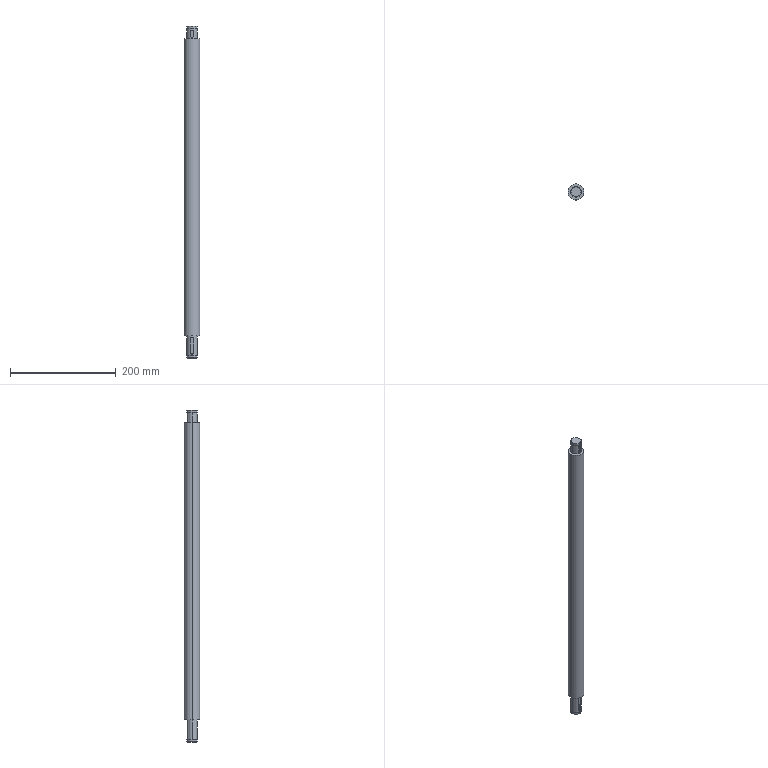Part | SolidWorks | features BaseBody 1 | 1 solid | 36 faces | box 30 x 30 x 627.444 mm | volume 416990 mm3 | cylinder 18 | plane 14 | cone 4 | commonest cylinder face diameters 20 x8 6 x4 18.35 x4 30 x2
STEP:
#1=CARTESIAN_POINT('',(9.,0.,-322.542));
#2=VERTEX_POINT('',#1);
#3=CARTESIAN_POINT('',(-9.,0.,-322.542));
#4=VERTEX_POINT('',#3);
#5=CARTESIAN_POINT('',(0.,0.,-322.542));
#6=DIRECTION('',(0.,0.,1.));
#7=DIRECTION('',(1.,0.,0.));
#8=AXIS2_PLACEMENT_3D('',#5,#6,#7);
#9=CIRCLE('',#8,9.);
#10=EDGE_CURVE('',#2,#4,#9,.T.);
#11=ORIENTED_EDGE('',*,*,#10,.T.);
#12=CARTESIAN_POINT('',(-10.,0.,-321.542));
#13=VERTEX_POINT('',#12);
#14=CARTESIAN_POINT('',(-9.5,0.,-322.042));
#15=DIRECTION('',(-0.7071,0.,0.7071));
#16=VECTOR('',#15,1000.);
#17=LINE('',#14,#16);
#18=EDGE_CURVE('',#4,#13,#17,.T.);
#19=ORIENTED_EDGE('',*,*,#18,.T.);
#20=CARTESIAN_POINT('',(10.,0.,-321.542));
#21=VERTEX_POINT('',#20);
#22=CARTESIAN_POINT('',(0.,0.,-321.542));
#23=DIRECTION('',(0.,0.,-1.));
#24=DIRECTION('',(1.,0.,0.));
#25=AXIS2_PLACEMENT_3D('',#22,#23,#24);
#26=CIRCLE('',#25,10.);
#27=EDGE_CURVE('',#13,#21,#26,.T.);
#28=ORIENTED_EDGE('',*,*,#27,.T.);
#29=CARTESIAN_POINT('',(9.5,0.,-322.042));
#30=DIRECTION('',(0.7071,0.,0.7071));
#31=VECTOR('',#30,1000.);
#32=LINE('',#29,#31);
#33=EDGE_CURVE('',#2,#21,#32,.T.);
#34=ORIENTED_EDGE('',*,*,#33,.F.);
#35=EDGE_LOOP('',(#11,#19,#28,#34));
#36=FACE_OUTER_BOUND('',#35,.T.);
#37=CARTESIAN_POINT('',(0.,0.,-322.042));
#38=DIRECTION('',(0.,0.,1.));
#39=DIRECTION('',(1.,0.,0.));
#40=AXIS2_PLACEMENT_3D('',#37,#38,#39);
#41=CONICAL_SURFACE('',#40,9.5,0.7854);
#42=ADVANCED_FACE('',(#36),#41,.T.);
#43=ORIENTED_EDGE('',*,*,#27,.F.);
#44=CARTESIAN_POINT('',(-10.,0.,-318.542));
#45=VERTEX_POINT('',#44);
#46=CARTESIAN_POINT('',(-10.,0.,-280.932));
#47=DIRECTION('',(0.,0.,1.));
#48=VECTOR('',#47,1000.);
#49=LINE('',#46,#48);
#50=EDGE_CURVE('',#13,#45,#49,.T.);
#51=ORIENTED_EDGE('',*,*,#50,.T.);
#52=CARTESIAN_POINT('',(10.,0.,-318.542));
#53=VERTEX_POINT('',#52);
#54=CARTESIAN_POINT('',(0.,0.,-318.542));
#55=DIRECTION('',(0.,0.,-1.));
#56=DIRECTION('',(1.,0.,0.));
#57=AXIS2_PLACEMENT_3D('',#54,#55,#56);
#58=CIRCLE('',#57,10.);
#59=EDGE_CURVE('',#45,#53,#58,.T.);
#60=ORIENTED_EDGE('',*,*,#59,.T.);
#61=CARTESIAN_POINT('',(10.,0.,-280.932));
#62=DIRECTION('',(0.,0.,1.));
#63=VECTOR('',#62,1000.);
#64=LINE('',#61,#63);
#65=EDGE_CURVE('',#21,#53,#64,.T.);
#66=ORIENTED_EDGE('',*,*,#65,.F.);
#67=EDGE_LOOP('',(#43,#51,#60,#66));
#68=FACE_OUTER_BOUND('',#67,.T.);
#69=CARTESIAN_POINT('',(0.,0.,-280.932));
#70=DIRECTION('',(0.,0.,1.));
#71=DIRECTION('',(1.,0.,0.));
#72=AXIS2_PLACEMENT_3D('',#69,#70,#71);
#73=CYLINDRICAL_SURFACE('',#72,10.);
#74=ADVANCED_FACE('',(#68),#73,.T.);
#75=CARTESIAN_POINT('',(9.175,0.,-317.342));
#76=VERTEX_POINT('',#75);
#77=CARTESIAN_POINT('',(-9.175,0.,-317.342));
#78=VERTEX_POINT('',#77);
#79=CARTESIAN_POINT('',(0.,0.,-317.342));
#80=DIRECTION('',(0.,0.,1.));
#81=DIRECTION('',(1.,0.,0.));
#82=AXIS2_PLACEMENT_3D('',#79,#80,#81);
#83=CIRCLE('',#82,9.175);
#84=EDGE_CURVE('',#76,#78,#83,.T.);
#85=ORIENTED_EDGE('',*,*,#84,.F.);
#86=CARTESIAN_POINT('',(9.175,0.,-318.542));
#87=VERTEX_POINT('',#86);
#88=CARTESIAN_POINT('',(9.175,0.,-317.942));
#89=DIRECTION('',(0.,0.,-1.));
#90=VECTOR('',#89,1000.);
#91=LINE('',#88,#90);
#92=EDGE_CURVE('',#76,#87,#91,.T.);
#93=ORIENTED_EDGE('',*,*,#92,.T.);
#94=CARTESIAN_POINT('',(-9.175,0.,-318.542));
#95=VERTEX_POINT('',#94);
#96=CARTESIAN_POINT('',(0.,0.,-318.542));
#97=DIRECTION('',(0.,0.,1.));
#98=DIRECTION('',(1.,0.,0.));
#99=AXIS2_PLACEMENT_3D('',#96,#97,#98);
#100=CIRCLE('',#99,9.175);
#101=EDGE_CURVE('',#87,#95,#100,.T.);
#102=ORIENTED_EDGE('',*,*,#101,.T.);
#103=CARTESIAN_POINT('',(-9.175,0.,-317.942));
#104=DIRECTION('',(0.,0.,-1.));
#105=VECTOR('',#104,1000.);
#106=LINE('',#103,#105);
#107=EDGE_CURVE('',#78,#95,#106,.T.);
#108=ORIENTED_EDGE('',*,*,#107,.F.);
#109=EDGE_LOOP('',(#85,#93,#102,#108));
#110=FACE_OUTER_BOUND('',#109,.T.);
#111=CARTESIAN_POINT('',(0.,0.,-317.942));
#112=DIRECTION('',(0.,0.,-1.));
#113=DIRECTION('',(-1.,0.,0.));
#114=AXIS2_PLACEMENT_3D('',#111,#112,#113);
#115=CYLINDRICAL_SURFACE('',#114,9.175);
#116=ADVANCED_FACE('',(#110),#115,.T.);
#117=CARTESIAN_POINT('',(10.,0.,-317.342));
#118=VERTEX_POINT('',#117);
#119=CARTESIAN_POINT('',(-10.,0.,-317.342));
#120=VERTEX_POINT('',#119);
#121=CARTESIAN_POINT('',(0.,0.,-317.342));
#122=DIRECTION('',(0.,0.,1.));
#123=DIRECTION('',(1.,0.,0.));
#124=AXIS2_PLACEMENT_3D('',#121,#122,#123);
#125=CIRCLE('',#124,10.);
#126=EDGE_CURVE('',#118,#120,#125,.T.);
#127=ORIENTED_EDGE('',*,*,#126,.T.);
#128=CARTESIAN_POINT('',(-10.,0.,-280.932));
#129=VERTEX_POINT('',#128);
#130=CARTESIAN_POINT('',(-10.,0.,-280.932));
#131=DIRECTION('',(0.,0.,1.));
#132=VECTOR('',#131,1000.);
#133=LINE('',#130,#132);
#134=EDGE_CURVE('',#120,#129,#133,.T.);
#135=ORIENTED_EDGE('',*,*,#134,.T.);
#136=CARTESIAN_POINT('',(10.,0.,-280.932));
#137=VERTEX_POINT('',#136);
#138=CARTESIAN_POINT('',(0.,0.,-280.932));
#139=DIRECTION('',(0.,0.,1.));
#140=DIRECTION('',(1.,0.,0.));
#141=AXIS2_PLACEMENT_3D('',#138,#139,#140);
#142=CIRCLE('',#141,10.);
#143=EDGE_CURVE('',#137,#129,#142,.T.);
#144=ORIENTED_EDGE('',*,*,#143,.F.);
#145=CARTESIAN_POINT('',(10.,0.,-280.932));
#146=DIRECTION('',(0.,0.,1.));
#147=VECTOR('',#146,1000.);
#148=LINE('',#145,#147);
#149=EDGE_CURVE('',#118,#137,#148,.T.);
#150=ORIENTED_EDGE('',*,*,#149,.F.);
#151=EDGE_LOOP('',(#127,#135,#144,#150));
#152=FACE_OUTER_BOUND('',#151,.T.);
#153=CARTESIAN_POINT('',(0.,0.,-280.932));
#154=DIRECTION('',(0.,0.,1.));
#155=DIRECTION('',(1.,0.,0.));
#156=AXIS2_PLACEMENT_3D('',#153,#154,#155);
#157=CYLINDRICAL_SURFACE('',#156,10.);
#158=ADVANCED_FACE('',(#152),#157,.T.);
#159=CARTESIAN_POINT('',(-9.5,0.,304.902));
#160=VERTEX_POINT('',#159);
#161=CARTESIAN_POINT('',(9.5,0.,304.902));
#162=VERTEX_POINT('',#161);
#163=CARTESIAN_POINT('',(0.,0.,304.902));
#164=DIRECTION('',(0.,0.,-1.));
#165=DIRECTION('',(-1.,0.,0.));
#166=AXIS2_PLACEMENT_3D('',#163,#164,#165);
#167=CIRCLE('',#166,9.5);
#168=EDGE_CURVE('',#160,#162,#167,.T.);
#169=ORIENTED_EDGE('',*,*,#168,.T.);
#170=CARTESIAN_POINT('',(10.,0.,304.402));
#171=VERTEX_POINT('',#170);
#172=CARTESIAN_POINT('',(9.75,0.,304.652));
#173=DIRECTION('',(0.7071,0.,-0.7071));
#174=VECTOR('',#173,1000.);
#175=LINE('',#172,#174);
#176=EDGE_CURVE('',#162,#171,#175,.T.);
#177=ORIENTED_EDGE('',*,*,#176,.T.);
#178=CARTESIAN_POINT('',(-10.,0.,304.402));
#179=VERTEX_POINT('',#178);
#180=CARTESIAN_POINT('',(0.,0.,304.402));
#181=DIRECTION('',(0.,0.,1.));
#182=DIRECTION('',(-1.,0.,0.));
#183=AXIS2_PLACEMENT_3D('',#180,#181,#182);
#184=CIRCLE('',#183,10.);
#185=EDGE_CURVE('',#171,#179,#184,.T.);
#186=ORIENTED_EDGE('',*,*,#185,.T.);
#187=CARTESIAN_POINT('',(-9.75,0.,304.652));
#188=DIRECTION('',(-0.7071,0.,-0.7071));
#189=VECTOR('',#188,1000.);
#190=LINE('',#187,#189);
#191=EDGE_CURVE('',#160,#179,#190,.T.);
#192=ORIENTED_EDGE('',*,*,#191,.F.);
#193=EDGE_LOOP('',(#169,#177,#186,#192));
#194=FACE_OUTER_BOUND('',#193,.T.);
#195=CARTESIAN_POINT('',(0.,0.,304.652));
#196=DIRECTION('',(0.,0.,-1.));
#197=DIRECTION('',(-1.,0.,0.));
#198=AXIS2_PLACEMENT_3D('',#195,#196,#197);
#199=CONICAL_SURFACE('',#198,9.75,0.7854);
#200=ADVANCED_FACE('',(#194),#199,.T.);
#201=ORIENTED_EDGE('',*,*,#185,.F.);
#202=CARTESIAN_POINT('',(10.,0.,300.902));
#203=VERTEX_POINT('',#202);
#204=CARTESIAN_POINT('',(10.,0.,280.932));
#205=DIRECTION('',(0.,0.,-1.));
#206=VECTOR('',#205,1000.);
#207=LINE('',#204,#206);
#208=EDGE_CURVE('',#171,#203,#207,.T.);
#209=ORIENTED_EDGE('',*,*,#208,.T.);
#210=CARTESIAN_POINT('',(-10.,0.,300.902));
#211=VERTEX_POINT('',#210);
#212=CARTESIAN_POINT('',(0.,0.,300.902));
#213=DIRECTION('',(0.,0.,1.));
#214=DIRECTION('',(-1.,0.,0.));
#215=AXIS2_PLACEMENT_3D('',#212,#213,#214);
#216=CIRCLE('',#215,10.);
#217=EDGE_CURVE('',#203,#211,#216,.T.);
#218=ORIENTED_EDGE('',*,*,#217,.T.);
#219=CARTESIAN_POINT('',(-10.,0.,280.932));
#220=DIRECTION('',(0.,0.,-1.));
#221=VECTOR('',#220,1000.);
#222=LINE('',#219,#221);
#223=EDGE_CURVE('',#179,#211,#222,.T.);
#224=ORIENTED_EDGE('',*,*,#223,.F.);
#225=EDGE_LOOP('',(#201,#209,#218,#224));
#226=FACE_OUTER_BOUND('',#225,.T.);
#227=CARTESIAN_POINT('',(0.,0.,280.932));
#228=DIRECTION('',(0.,0.,-1.));
#229=DIRECTION('',(-1.,0.,0.));
#230=AXIS2_PLACEMENT_3D('',#227,#228,#229);
#231=CYLINDRICAL_SURFACE('',#230,10.);
#232=ADVANCED_FACE('',(#226),#231,.T.);
#233=CARTESIAN_POINT('',(-9.175,0.,299.702));
#234=VERTEX_POINT('',#233);
#235=CARTESIAN_POINT('',(9.175,0.,299.702));
#236=VERTEX_POINT('',#235);
#237=CARTESIAN_POINT('',(0.,0.,299.702));
#238=DIRECTION('',(0.,0.,-1.));
#239=DIRECTION('',(1.,0.,0.));
#240=AXIS2_PLACEMENT_3D('',#237,#238,#239);
#241=CIRCLE('',#240,9.175);
#242=EDGE_CURVE('',#234,#236,#241,.T.);
#243=ORIENTED_EDGE('',*,*,#242,.F.);
#244=CARTESIAN_POINT('',(-9.175,0.,300.902));
#245=VERTEX_POINT('',#244);
#246=CARTESIAN_POINT('',(-9.175,0.,300.302));
#247=DIRECTION('',(0.,0.,1.));
#248=VECTOR('',#247,1000.);
#249=LINE('',#246,#248);
#250=EDGE_CURVE('',#234,#245,#249,.T.);
#251=ORIENTED_EDGE('',*,*,#250,.T.);
#252=CARTESIAN_POINT('',(9.175,0.,300.902));
#253=VERTEX_POINT('',#252);
#254=CARTESIAN_POINT('',(0.,0.,300.902));
#255=DIRECTION('',(0.,0.,-1.));
#256=DIRECTION('',(1.,0.,0.));
#257=AXIS2_PLACEMENT_3D('',#254,#255,#256);
#258=CIRCLE('',#257,9.175);
#259=EDGE_CURVE('',#245,#253,#258,.T.);
#260=ORIENTED_EDGE('',*,*,#259,.T.);
#261=CARTESIAN_POINT('',(9.175,0.,300.302));
#262=DIRECTION('',(0.,0.,1.));
#263=VECTOR('',#262,1000.);
#264=LINE('',#261,#263);
#265=EDGE_CURVE('',#236,#253,#264,.T.);
#266=ORIENTED_EDGE('',*,*,#265,.F.);
#267=EDGE_LOOP('',(#243,#251,#260,#266));
#268=FACE_OUTER_BOUND('',#267,.T.);
#269=CARTESIAN_POINT('',(0.,0.,300.302));
#270=DIRECTION('',(0.,0.,1.));
#271=DIRECTION('',(1.,0.,0.));
#272=AXIS2_PLACEMENT_3D('',#269,#270,#271);
#273=CYLINDRICAL_SURFACE('',#272,9.175);
#274=ADVANCED_FACE('',(#268),#273,.T.);
#275=CARTESIAN_POINT('',(-10.,0.,299.702));
#276=VERTEX_POINT('',#275);
#277=CARTESIAN_POINT('',(10.,0.,299.702));
#278=VERTEX_POINT('',#277);
#279=CARTESIAN_POINT('',(0.,0.,299.702));
#280=DIRECTION('',(0.,0.,-1.));
#281=DIRECTION('',(-1.,0.,0.));
#282=AXIS2_PLACEMENT_3D('',#279,#280,#281);
#283=CIRCLE('',#282,10.);
#284=EDGE_CURVE('',#276,#278,#283,.T.);
#285=ORIENTED_EDGE('',*,*,#284,.T.);
#286=CARTESIAN_POINT('',(10.,0.,280.932));
#287=VERTEX_POINT('',#286);
#288=CARTESIAN_POINT('',(10.,0.,280.932));
#289=DIRECTION('',(0.,0.,-1.));
#290=VECTOR('',#289,1000.);
#291=LINE('',#288,#290);
#292=EDGE_CURVE('',#278,#287,#291,.T.);
#293=ORIENTED_EDGE('',*,*,#292,.T.);
#294=CARTESIAN_POINT('',(-10.,0.,280.932));
#295=VERTEX_POINT('',#294);
#296=CARTESIAN_POINT('',(0.,0.,280.932));
#297=DIRECTION('',(0.,0.,-1.));
#298=DIRECTION('',(-1.,0.,0.));
#299=AXIS2_PLACEMENT_3D('',#296,#297,#298);
#300=CIRCLE('',#299,10.);
#301=EDGE_CURVE('',#295,#287,#300,.T.);
#302=ORIENTED_EDGE('',*,*,#301,.F.);
#303=CARTESIAN_POINT('',(-10.,0.,280.932));
#304=DIRECTION('',(0.,0.,-1.));
#305=VECTOR('',#304,1000.);
#306=LINE('',#303,#305);
#307=EDGE_CURVE('',#276,#295,#306,.T.);
#308=ORIENTED_EDGE('',*,*,#307,.F.);
#309=EDGE_LOOP('',(#285,#293,#302,#308));
#310=FACE_OUTER_BOUND('',#309,.T.);
#311=CARTESIAN_POINT('',(0.,0.,280.932));
#312=DIRECTION('',(0.,0.,-1.));
#313=DIRECTION('',(-1.,0.,0.));
#314=AXIS2_PLACEMENT_3D('',#311,#312,#313);
#315=CYLINDRICAL_SURFACE('',#314,10.);
#316=ADVANCED_FACE('',(#310),#315,.T.);
#317=CARTESIAN_POINT('',(15.,0.,280.932));
#318=VERTEX_POINT('',#317);
#319=CARTESIAN_POINT('',(-15.,0.,280.932));
#320=VERTEX_POINT('',#319);
#321=CARTESIAN_POINT('',(0.,0.,280.932));
#322=DIRECTION('',(0.,0.,1.));
#323=DIRECTION('',(-1.,0.,0.));
#324=AXIS2_PLACEMENT_3D('',#321,#322,#323);
#325=CIRCLE('',#324,15.);
#326=EDGE_CURVE('',#318,#320,#325,.T.);
#327=ORIENTED_EDGE('',*,*,#326,.F.);
#328=CARTESIAN_POINT('',(15.,0.,-280.932));
#329=VERTEX_POINT('',#328);
#330=CARTESIAN_POINT('',(15.,0.,0.));
#331=DIRECTION('',(0.,0.,-1.));
#332=VECTOR('',#331,1000.);
#333=LINE('',#330,#332);
#334=EDGE_CURVE('',#318,#329,#333,.T.);
#335=ORIENTED_EDGE('',*,*,#334,.T.);
#336=CARTESIAN_POINT('',(-15.,0.,-280.932));
#337=VERTEX_POINT('',#336);
#338=CARTESIAN_POINT('',(0.,0.,-280.932));
#339=DIRECTION('',(0.,0.,-1.));
#340=DIRECTION('',(-1.,0.,0.));
#341=AXIS2_PLACEMENT_3D('',#338,#339,#340);
#342=CIRCLE('',#341,15.);
#343=EDGE_CURVE('',#337,#329,#342,.T.);
#344=ORIENTED_EDGE('',*,*,#343,.F.);
#345=CARTESIAN_POINT('',(-15.,0.,0.));
#346=DIRECTION('',(0.,0.,-1.));
#347=VECTOR('',#346,1000.);
#348=LINE('',#345,#347);
#349=EDGE_CURVE('',#320,#337,#348,.T.);
#350=ORIENTED_EDGE('',*,*,#349,.F.);
#351=EDGE_LOOP('',(#327,#335,#344,#350));
#352=FACE_OUTER_BOUND('',#351,.T.);
#353=CARTESIAN_POINT('',(0.,0.,0.));
#354=DIRECTION('',(0.,0.,-1.));
#355=DIRECTION('',(-1.,0.,0.));
#356=AXIS2_PLACEMENT_3D('',#353,#354,#355);
#357=CYLINDRICAL_SURFACE('',#356,15.);
#358=ADVANCED_FACE('',(#352),#357,.T.);
#359=ORIENTED_EDGE('',*,*,#10,.F.);
#360=CARTESIAN_POINT('',(0.,0.,-322.542));
#361=DIRECTION('',(0.,0.,1.));
#362=DIRECTION('',(1.,0.,0.));
#363=AXIS2_PLACEMENT_3D('',#360,#361,#362);
#364=CIRCLE('',#363,9.);
#365=EDGE_CURVE('',#4,#2,#364,.T.);
#366=ORIENTED_EDGE('',*,*,#365,.F.);
#367=EDGE_LOOP('',(#359,#366));
#368=FACE_OUTER_BOUND('',#367,.T.);
#369=CARTESIAN_POINT('',(0.,0.,-322.542));
#370=DIRECTION('',(0.,0.,1.));
#371=DIRECTION('',(1.,0.,0.));
#372=AXIS2_PLACEMENT_3D('',#369,#370,#371);
#373=PLANE('',#372);
#374=ADVANCED_FACE('',(#368),#373,.F.);
#375=CARTESIAN_POINT('',(0.,0.,-317.342));
#376=DIRECTION('',(0.,0.,1.));
#377=DIRECTION('',(1.,0.,0.));
#378=AXIS2_PLACEMENT_3D('',#375,#376,#377);
#379=CIRCLE('',#378,9.175);
#380=EDGE_CURVE('',#78,#76,#379,.T.);
#381=ORIENTED_EDGE('',*,*,#380,.T.);
#382=ORIENTED_EDGE('',*,*,#84,.T.);
#383=EDGE_LOOP('',(#381,#382));
#384=FACE_BOUND('',#383,.T.);
#385=ORIENTED_EDGE('',*,*,#126,.F.);
#386=CARTESIAN_POINT('',(0.,0.,-317.342));
#387=DIRECTION('',(0.,0.,1.));
#388=DIRECTION('',(1.,0.,0.));
#389=AXIS2_PLACEMENT_3D('',#386,#387,#388);
#390=CIRCLE('',#389,10.);
#391=EDGE_CURVE('',#120,#118,#390,.T.);
#392=ORIENTED_EDGE('',*,*,#391,.F.);
#393=EDGE_LOOP('',(#385,#392));
#394=FACE_OUTER_BOUND('',#393,.T.);
#395=CARTESIAN_POINT('',(-9.175,0.,-317.342));
#396=DIRECTION('',(0.,0.,1.));
#397=DIRECTION('',(1.,0.,0.));
#398=AXIS2_PLACEMENT_3D('',#395,#396,#397);
#399=PLANE('',#398);
#400=ADVANCED_FACE('',(#384,#394),#399,.F.);
#401=CARTESIAN_POINT('',(0.,0.,-318.542));
#402=DIRECTION('',(0.,0.,1.));
#403=DIRECTION('',(1.,0.,0.));
#404=AXIS2_PLACEMENT_3D('',#401,#402,#403);
#405=CIRCLE('',#404,9.175);
#406=EDGE_CURVE('',#95,#87,#405,.T.);
#407=ORIENTED_EDGE('',*,*,#406,.F.);
#408=ORIENTED_EDGE('',*,*,#101,.F.);
#409=EDGE_LOOP('',(#407,#408));
#410=FACE_BOUND('',#409,.T.);
#411=CARTESIAN_POINT('',(0.,0.,-318.542));
#412=DIRECTION('',(0.,0.,-1.));
#413=DIRECTION('',(1.,0.,0.));
#414=AXIS2_PLACEMENT_3D('',#411,#412,#413);
#415=CIRCLE('',#414,10.);
#416=EDGE_CURVE('',#53,#45,#415,.T.);
#417=ORIENTED_EDGE('',*,*,#416,.F.);
#418=ORIENTED_EDGE('',*,*,#59,.F.);
#419=EDGE_LOOP('',(#417,#418));
#420=FACE_OUTER_BOUND('',#419,.T.);
#421=CARTESIAN_POINT('',(-14.987,0.,-318.542));
#422=DIRECTION('',(0.,0.,-1.));
#423=DIRECTION('',(-1.,0.,0.));
#424=AXIS2_PLACEMENT_3D('',#421,#422,#423);
#425=PLANE('',#424);
#426=ADVANCED_FACE('',(#410,#420),#425,.F.);
#427=CARTESIAN_POINT('',(3.,-9.539,-286.137));
#428=VERTEX_POINT('',#427);
#429=CARTESIAN_POINT('',(3.,-9.539,-312.137));
#430=VERTEX_POINT('',#429);
#431=CARTESIAN_POINT('',(3.,-9.539,-280.932));
#432=DIRECTION('',(0.,0.,-1.));
#433=VECTOR('',#432,1000.);
#434=LINE('',#431,#433);
#435=EDGE_CURVE('',#428,#430,#434,.T.);
#436=ORIENTED_EDGE('',*,*,#435,.F.);
#437=CARTESIAN_POINT('',(3.,-7.5,-286.137));
#438=VERTEX_POINT('',#437);
#439=CARTESIAN_POINT('',(3.,-10.,-286.137));
#440=DIRECTION('',(0.,1.,0.));
#441=VECTOR('',#440,1000.);
#442=LINE('',#439,#441);
#443=EDGE_CURVE('',#428,#438,#442,.T.);
#444=ORIENTED_EDGE('',*,*,#443,.T.);
#445=CARTESIAN_POINT('',(3.,-7.5,-312.137));
#446=VERTEX_POINT('',#445);
#447=CARTESIAN_POINT('',(3.,-7.5,-286.137));
#448=DIRECTION('',(0.,0.,-1.));
#449=VECTOR('',#448,1000.);
#450=LINE('',#447,#449);
#451=EDGE_CURVE('',#438,#446,#450,.T.);
#452=ORIENTED_EDGE('',*,*,#451,.T.);
#453=CARTESIAN_POINT('',(3.,-10.,-312.137));
#454=DIRECTION('',(0.,1.,0.));
#455=VECTOR('',#454,1000.);
#456=LINE('',#453,#455);
#457=EDGE_CURVE('',#430,#446,#456,.T.);
#458=ORIENTED_EDGE('',*,*,#457,.F.);
#459=EDGE_LOOP('',(#436,#444,#452,#458));
#460=FACE_OUTER_BOUND('',#459,.T.);
#461=CARTESIAN_POINT('',(3.,-10.,-286.137));
#462=DIRECTION('',(1.,0.,0.));
#463=DIRECTION('',(0.,0.,-1.));
#464=AXIS2_PLACEMENT_3D('',#461,#462,#463);
#465=PLANE('',#464);
#466=ADVANCED_FACE('',(#460),#465,.F.);
#467=CARTESIAN_POINT('',(-3.,-9.539,-312.137));
#468=VERTEX_POINT('',#467);
#469=CARTESIAN_POINT('',(3.,-9.539,-312.137));
#470=CARTESIAN_POINT('',(3.,-9.539,-312.336));
#471=CARTESIAN_POINT('',(2.98,-9.546,-312.532));
#472=CARTESIAN_POINT('',(2.904,-9.569,-312.917));
#473=CARTESIAN_POINT('',(2.845,-9.587,-313.108));
#474=CARTESIAN_POINT('',(2.695,-9.63,-313.47));
#475=CARTESIAN_POINT('',(2.602,-9.656,-313.642));
#476=CARTESIAN_POINT('',(2.385,-9.712,-313.967));
#477=CARTESIAN_POINT('',(2.259,-9.742,-314.12));
#478=CARTESIAN_POINT('',(1.847,-9.832,-314.533));
#479=CARTESIAN_POINT('',(1.515,-9.891,-314.756));
#480=CARTESIAN_POINT('',(0.9743,-9.954,-314.981));
#481=CARTESIAN_POINT('',(0.7844,-9.971,-315.039));
#482=CARTESIAN_POINT('',(0.396,-9.994,-315.117));
#483=CARTESIAN_POINT('',(0.1993,-10.,-315.137));
#484=CARTESIAN_POINT('',(-0.1994,-10.,-315.137));
#485=CARTESIAN_POINT('',(-0.3951,-9.994,-315.117));
#486=CARTESIAN_POINT('',(-0.7799,-9.971,-315.04));
#487=CARTESIAN_POINT('',(-0.971,-9.954,-314.982));
#488=CARTESIAN_POINT('',(-1.334,-9.912,-314.831));
#489=CARTESIAN_POINT('',(-1.505,-9.887,-314.739));
#490=CARTESIAN_POINT('',(-1.831,-9.832,-314.522));
#491=CARTESIAN_POINT('',(-1.984,-9.802,-314.396));
#492=CARTESIAN_POINT('',(-2.396,-9.713,-313.984));
#493=CARTESIAN_POINT('',(-2.619,-9.652,-313.651));
#494=CARTESIAN_POINT('',(-2.844,-9.587,-313.111));
#495=CARTESIAN_POINT('',(-2.902,-9.57,-312.921));
#496=CARTESIAN_POINT('',(-2.98,-9.546,-312.533));
#497=CARTESIAN_POINT('',(-3.,-9.539,-312.336));
#498=CARTESIAN_POINT('',(-3.,-9.539,-312.137));
#499=B_SPLINE_CURVE_WITH_KNOTS('',3,(#469,#470,#471,#472,#473,#474,#475,#476,#477,#478,#479,#480,#481,#482,#483,#484,#485,#486,#487,#488,#489,#490,#491,#492,#493,#494,#495,#496,#497,#498),.UNSPECIFIED.,.F.,.F.,(4,2,2,2,2,2,2,2,2,2,2,2,2,2,4),(0.,0.0005892,0.001178,0.001768,0.002357,0.003535,0.004125,0.004714,0.005303,0.005892,0.006482,0.007071,0.008249,0.008838,0.009428),.UNSPECIFIED.);
#500=EDGE_CURVE('',#430,#468,#499,.T.);
#501=ORIENTED_EDGE('',*,*,#500,.F.);
#502=ORIENTED_EDGE('',*,*,#457,.T.);
#503=CARTESIAN_POINT('',(-3.,-7.5,-312.137));
#504=VERTEX_POINT('',#503);
#505=CARTESIAN_POINT('',(0.,-7.5,-312.137));
#506=DIRECTION('',(0.,1.,0.));
#507=DIRECTION('',(1.,0.,0.));
#508=AXIS2_PLACEMENT_3D('',#505,#506,#507);
#509=CIRCLE('',#508,3.);
#510=EDGE_CURVE('',#446,#504,#509,.T.);
#511=ORIENTED_EDGE('',*,*,#510,.T.);
#512=CARTESIAN_POINT('',(-3.,-10.,-312.137));
#513=DIRECTION('',(0.,1.,0.));
#514=VECTOR('',#513,1000.);
#515=LINE('',#512,#514);
#516=EDGE_CURVE('',#468,#504,#515,.T.);
#517=ORIENTED_EDGE('',*,*,#516,.F.);
#518=EDGE_LOOP('',(#501,#502,#511,#517));
#519=FACE_OUTER_BOUND('',#518,.T.);
#520=CARTESIAN_POINT('',(0.,-10.,-312.137));
#521=DIRECTION('',(0.,-1.,0.));
#522=DIRECTION('',(1.,0.,0.));
#523=AXIS2_PLACEMENT_3D('',#520,#521,#522);
#524=CYLINDRICAL_SURFACE('',#523,3.);
#525=ADVANCED_FACE('',(#519),#524,.F.);
#526=CARTESIAN_POINT('',(-3.,-9.539,-286.137));
#527=VERTEX_POINT('',#526);
#528=CARTESIAN_POINT('',(-3.,-9.539,-280.932));
#529=DIRECTION('',(0.,0.,1.));
#530=VECTOR('',#529,1000.);
#531=LINE('',#528,#530);
#532=EDGE_CURVE('',#468,#527,#531,.T.);
#533=ORIENTED_EDGE('',*,*,#532,.F.);
#534=ORIENTED_EDGE('',*,*,#516,.T.);
#535=CARTESIAN_POINT('',(-3.,-7.5,-286.137));
#536=VERTEX_POINT('',#535);
#537=CARTESIAN_POINT('',(-3.,-7.5,-312.137));
#538=DIRECTION('',(0.,0.,1.));
#539=VECTOR('',#538,1000.);
#540=LINE('',#537,#539);
#541=EDGE_CURVE('',#504,#536,#540,.T.);
#542=ORIENTED_EDGE('',*,*,#541,.T.);
#543=CARTESIAN_POINT('',(-3.,-10.,-286.137));
#544=DIRECTION('',(0.,1.,0.));
#545=VECTOR('',#544,1000.);
#546=LINE('',#543,#545);
#547=EDGE_CURVE('',#527,#536,#546,.T.);
#548=ORIENTED_EDGE('',*,*,#547,.F.);
#549=EDGE_LOOP('',(#533,#534,#542,#548));
#550=FACE_OUTER_BOUND('',#549,.T.);
#551=CARTESIAN_POINT('',(-3.,-10.,-312.137));
#552=DIRECTION('',(-1.,0.,0.));
#553=DIRECTION('',(0.,0.,1.));
#554=AXIS2_PLACEMENT_3D('',#551,#552,#553);
#555=PLANE('',#554);
#556=ADVANCED_FACE('',(#550),#555,.F.);
#557=ORIENTED_EDGE('',*,*,#443,.F.);
#558=CARTESIAN_POINT('',(-3.,-9.539,-286.137));
#559=CARTESIAN_POINT('',(-3.,-9.539,-285.938));
#560=CARTESIAN_POINT('',(-2.98,-9.546,-285.742));
#561=CARTESIAN_POINT('',(-2.904,-9.569,-285.357));
#562=CARTESIAN_POINT('',(-2.845,-9.587,-285.166));
#563=CARTESIAN_POINT('',(-2.695,-9.63,-284.804));
#564=CARTESIAN_POINT('',(-2.602,-9.656,-284.632));
#565=CARTESIAN_POINT('',(-2.385,-9.712,-284.307));
#566=CARTESIAN_POINT('',(-2.259,-9.742,-284.154));
#567=CARTESIAN_POINT('',(-1.847,-9.832,-283.741));
#568=CARTESIAN_POINT('',(-1.515,-9.891,-283.518));
#569=CARTESIAN_POINT('',(-0.9743,-9.954,-283.293));
#570=CARTESIAN_POINT('',(-0.7844,-9.971,-283.235));
#571=CARTESIAN_POINT('',(-0.396,-9.994,-283.157));
#572=CARTESIAN_POINT('',(-0.1993,-10.,-283.137));
#573=CARTESIAN_POINT('',(0.1994,-10.,-283.137));
#574=CARTESIAN_POINT('',(0.3951,-9.994,-283.157));
#575=CARTESIAN_POINT('',(0.7799,-9.971,-283.234));
#576=CARTESIAN_POINT('',(0.971,-9.954,-283.292));
#577=CARTESIAN_POINT('',(1.334,-9.912,-283.443));
#578=CARTESIAN_POINT('',(1.505,-9.887,-283.535));
#579=CARTESIAN_POINT('',(1.831,-9.832,-283.752));
#580=CARTESIAN_POINT('',(1.984,-9.802,-283.878));
#581=CARTESIAN_POINT('',(2.396,-9.713,-284.29));
#582=CARTESIAN_POINT('',(2.619,-9.652,-284.623));
#583=CARTESIAN_POINT('',(2.844,-9.587,-285.163));
#584=CARTESIAN_POINT('',(2.902,-9.57,-285.353));
#585=CARTESIAN_POINT('',(2.98,-9.546,-285.741));
#586=CARTESIAN_POINT('',(3.,-9.539,-285.938));
#587=CARTESIAN_POINT('',(3.,-9.539,-286.137));
#588=B_SPLINE_CURVE_WITH_KNOTS('',3,(#558,#559,#560,#561,#562,#563,#564,#565,#566,#567,#568,#569,#570,#571,#572,#573,#574,#575,#576,#577,#578,#579,#580,#581,#582,#583,#584,#585,#586,#587),.UNSPECIFIED.,.F.,.F.,(4,2,2,2,2,2,2,2,2,2,2,2,2,2,4),(0.,0.0005892,0.001178,0.001768,0.002357,0.003535,0.004125,0.004714,0.005303,0.005892,0.006482,0.007071,0.008249,0.008838,0.009428),.UNSPECIFIED.);
#589=EDGE_CURVE('',#527,#428,#588,.T.);
#590=ORIENTED_EDGE('',*,*,#589,.F.);
#591=ORIENTED_EDGE('',*,*,#547,.T.);
#592=CARTESIAN_POINT('',(0.,-7.5,-286.137));
#593=DIRECTION('',(0.,1.,0.));
#594=DIRECTION('',(-1.,0.,0.));
#595=AXIS2_PLACEMENT_3D('',#592,#593,#594);
#596=CIRCLE('',#595,3.);
#597=EDGE_CURVE('',#536,#438,#596,.T.);
#598=ORIENTED_EDGE('',*,*,#597,.T.);
#599=EDGE_LOOP('',(#557,#590,#591,#598));
#600=FACE_OUTER_BOUND('',#599,.T.);
#601=CARTESIAN_POINT('',(0.,-10.,-286.137));
#602=DIRECTION('',(0.,-1.,0.));
#603=DIRECTION('',(-1.,0.,0.));
#604=AXIS2_PLACEMENT_3D('',#601,#602,#603);
#605=CYLINDRICAL_SURFACE('',#604,3.);
#606=ADVANCED_FACE('',(#600),#605,.F.);
#607=ORIENTED_EDGE('',*,*,#510,.F.);
#608=ORIENTED_EDGE('',*,*,#451,.F.);
#609=ORIENTED_EDGE('',*,*,#597,.F.);
#610=ORIENTED_EDGE('',*,*,#541,.F.);
#611=EDGE_LOOP('',(#607,#608,#609,#610));
#612=FACE_OUTER_BOUND('',#611,.T.);
#613=CARTESIAN_POINT('',(0.,-7.5,-313.17));
#614=DIRECTION('',(0.,1.,0.));
#615=DIRECTION('',(1.,0.,0.));
#616=AXIS2_PLACEMENT_3D('',#613,#614,#615);
#617=PLANE('',#616);
#618=ADVANCED_FACE('',(#612),#617,.F.);
#619=ORIENTED_EDGE('',*,*,#168,.F.);
#620=CARTESIAN_POINT('',(0.,0.,304.902));
#621=DIRECTION('',(0.,0.,-1.));
#622=DIRECTION('',(-1.,0.,0.));
#623=AXIS2_PLACEMENT_3D('',#620,#621,#622);
#624=CIRCLE('',#623,9.5);
#625=EDGE_CURVE('',#162,#160,#624,.T.);
#626=ORIENTED_EDGE('',*,*,#625,.F.);
#627=EDGE_LOOP('',(#619,#626));
#628=FACE_OUTER_BOUND('',#627,.T.);
#629=CARTESIAN_POINT('',(0.,0.,304.902));
#630=DIRECTION('',(0.,0.,1.));
#631=DIRECTION('',(1.,0.,0.));
#632=AXIS2_PLACEMENT_3D('',#629,#630,#631);
#633=PLANE('',#632);
#634=ADVANCED_FACE('',(#628),#633,.T.);
#635=CARTESIAN_POINT('',(0.,0.,300.902));
#636=DIRECTION('',(0.,0.,-1.));
#637=DIRECTION('',(1.,0.,0.));
#638=AXIS2_PLACEMENT_3D('',#635,#636,#637);
#639=CIRCLE('',#638,9.175);
#640=EDGE_CURVE('',#253,#245,#639,.T.);
#641=ORIENTED_EDGE('',*,*,#640,.F.);
#642=ORIENTED_EDGE('',*,*,#259,.F.);
#643=EDGE_LOOP('',(#641,#642));
#644=FACE_BOUND('',#643,.T.);
#645=CARTESIAN_POINT('',(0.,0.,300.902));
#646=DIRECTION('',(0.,0.,1.));
#647=DIRECTION('',(-1.,0.,0.));
#648=AXIS2_PLACEMENT_3D('',#645,#646,#647);
#649=CIRCLE('',#648,10.);
#650=EDGE_CURVE('',#211,#203,#649,.T.);
#651=ORIENTED_EDGE('',*,*,#650,.F.);
#652=ORIENTED_EDGE('',*,*,#217,.F.);
#653=EDGE_LOOP('',(#651,#652));
#654=FACE_OUTER_BOUND('',#653,.T.);
#655=CARTESIAN_POINT('',(11.292,0.,300.902));
#656=DIRECTION('',(0.,0.,1.));
#657=DIRECTION('',(1.,0.,0.));
#658=AXIS2_PLACEMENT_3D('',#655,#656,#657);
#659=PLANE('',#658);
#660=ADVANCED_FACE('',(#644,#654),#659,.F.);
#661=CARTESIAN_POINT('',(0.,0.,299.702));
#662=DIRECTION('',(0.,0.,-1.));
#663=DIRECTION('',(1.,0.,0.));
#664=AXIS2_PLACEMENT_3D('',#661,#662,#663);
#665=CIRCLE('',#664,9.175);
#666=EDGE_CURVE('',#236,#234,#665,.T.);
#667=ORIENTED_EDGE('',*,*,#666,.T.);
#668=ORIENTED_EDGE('',*,*,#242,.T.);
#669=EDGE_LOOP('',(#667,#668));
#670=FACE_BOUND('',#669,.T.);
#671=ORIENTED_EDGE('',*,*,#284,.F.);
#672=CARTESIAN_POINT('',(0.,0.,299.702));
#673=DIRECTION('',(0.,0.,-1.));
#674=DIRECTION('',(-1.,0.,0.));
#675=AXIS2_PLACEMENT_3D('',#672,#673,#674);
#676=CIRCLE('',#675,10.);
#677=EDGE_CURVE('',#278,#276,#676,.T.);
#678=ORIENTED_EDGE('',*,*,#677,.F.);
#679=EDGE_LOOP('',(#671,#678));
#680=FACE_OUTER_BOUND('',#679,.T.);
#681=CARTESIAN_POINT('',(9.175,0.,299.702));
#682=DIRECTION('',(0.,0.,-1.));
#683=DIRECTION('',(0.,-1.,0.));
#684=AXIS2_PLACEMENT_3D('',#681,#682,#683);
#685=PLANE('',#684);
#686=ADVANCED_FACE('',(#670,#680),#685,.F.);
#687=CARTESIAN_POINT('',(-3.,-9.539,286.317));
#688=VERTEX_POINT('',#687);
#689=CARTESIAN_POINT('',(-3.,-9.539,294.317));
#690=VERTEX_POINT('',#689);
#691=CARTESIAN_POINT('',(-3.,-9.539,280.932));
#692=DIRECTION('',(0.,0.,1.));
#693=VECTOR('',#692,1000.);
#694=LINE('',#691,#693);
#695=EDGE_CURVE('',#688,#690,#694,.T.);
#696=ORIENTED_EDGE('',*,*,#695,.F.);
#697=CARTESIAN_POINT('',(-3.,-7.5,286.317));
#698=VERTEX_POINT('',#697);
#699=CARTESIAN_POINT('',(-3.,-10.,286.317));
#700=DIRECTION('',(0.,1.,0.));
#701=VECTOR('',#700,1000.);
#702=LINE('',#699,#701);
#703=EDGE_CURVE('',#688,#698,#702,.T.);
#704=ORIENTED_EDGE('',*,*,#703,.T.);
#705=CARTESIAN_POINT('',(-3.,-7.5,294.317));
#706=VERTEX_POINT('',#705);
#707=CARTESIAN_POINT('',(-3.,-7.5,286.317));
#708=DIRECTION('',(0.,0.,1.));
#709=VECTOR('',#708,1000.);
#710=LINE('',#707,#709);
#711=EDGE_CURVE('',#698,#706,#710,.T.);
#712=ORIENTED_EDGE('',*,*,#711,.T.);
#713=CARTESIAN_POINT('',(-3.,-10.,294.317));
#714=DIRECTION('',(0.,1.,0.));
#715=VECTOR('',#714,1000.);
#716=LINE('',#713,#715);
#717=EDGE_CURVE('',#690,#706,#716,.T.);
#718=ORIENTED_EDGE('',*,*,#717,.F.);
#719=EDGE_LOOP('',(#696,#704,#712,#718));
#720=FACE_OUTER_BOUND('',#719,.T.);
#721=CARTESIAN_POINT('',(-3.,-10.,286.317));
#722=DIRECTION('',(-1.,0.,0.));
#723=DIRECTION('',(0.,0.,1.));
#724=AXIS2_PLACEMENT_3D('',#721,#722,#723);
#725=PLANE('',#724);
#726=ADVANCED_FACE('',(#720),#725,.F.);
#727=CARTESIAN_POINT('',(3.,-9.539,294.317));
#728=VERTEX_POINT('',#727);
#729=CARTESIAN_POINT('',(-3.,-9.539,294.317));
#730=CARTESIAN_POINT('',(-3.,-9.539,294.516));
#731=CARTESIAN_POINT('',(-2.98,-9.546,294.712));
#732=CARTESIAN_POINT('',(-2.904,-9.569,295.097));
#733=CARTESIAN_POINT('',(-2.845,-9.587,295.288));
#734=CARTESIAN_POINT('',(-2.695,-9.63,295.65));
#735=CARTESIAN_POINT('',(-2.602,-9.656,295.822));
#736=CARTESIAN_POINT('',(-2.385,-9.712,296.147));
#737=CARTESIAN_POINT('',(-2.259,-9.742,296.3));
#738=CARTESIAN_POINT('',(-1.847,-9.832,296.713));
#739=CARTESIAN_POINT('',(-1.515,-9.891,296.936));
#740=CARTESIAN_POINT('',(-0.9743,-9.954,297.161));
#741=CARTESIAN_POINT('',(-0.7844,-9.971,297.219));
#742=CARTESIAN_POINT('',(-0.396,-9.994,297.297));
#743=CARTESIAN_POINT('',(-0.1993,-10.,297.317));
#744=CARTESIAN_POINT('',(0.1994,-10.,297.317));
#745=CARTESIAN_POINT('',(0.3951,-9.994,297.297));
#746=CARTESIAN_POINT('',(0.7799,-9.971,297.22));
#747=CARTESIAN_POINT('',(0.971,-9.954,297.162));
#748=CARTESIAN_POINT('',(1.334,-9.912,297.011));
#749=CARTESIAN_POINT('',(1.505,-9.887,296.919));
#750=CARTESIAN_POINT('',(1.831,-9.832,296.702));
#751=CARTESIAN_POINT('',(1.984,-9.802,296.576));
#752=CARTESIAN_POINT('',(2.396,-9.713,296.164));
#753=CARTESIAN_POINT('',(2.619,-9.652,295.831));
#754=CARTESIAN_POINT('',(2.844,-9.587,295.291));
#755=CARTESIAN_POINT('',(2.902,-9.57,295.101));
#756=CARTESIAN_POINT('',(2.98,-9.546,294.713));
#757=CARTESIAN_POINT('',(3.,-9.539,294.516));
#758=CARTESIAN_POINT('',(3.,-9.539,294.317));
#759=B_SPLINE_CURVE_WITH_KNOTS('',3,(#729,#730,#731,#732,#733,#734,#735,#736,#737,#738,#739,#740,#741,#742,#743,#744,#745,#746,#747,#748,#749,#750,#751,#752,#753,#754,#755,#756,#757,#758),.UNSPECIFIED.,.F.,.F.,(4,2,2,2,2,2,2,2,2,2,2,2,2,2,4),(0.,0.0005892,0.001178,0.001768,0.002357,0.003535,0.004125,0.004714,0.005303,0.005892,0.006482,0.007071,0.008249,0.008838,0.009428),.UNSPECIFIED.);
#760=EDGE_CURVE('',#690,#728,#759,.T.);
#761=ORIENTED_EDGE('',*,*,#760,.F.);
#762=ORIENTED_EDGE('',*,*,#717,.T.);
#763=CARTESIAN_POINT('',(3.,-7.5,294.317));
#764=VERTEX_POINT('',#763);
#765=CARTESIAN_POINT('',(0.,-7.5,294.317));
#766=DIRECTION('',(0.,1.,0.));
#767=DIRECTION('',(-1.,0.,0.));
#768=AXIS2_PLACEMENT_3D('',#765,#766,#767);
#769=CIRCLE('',#768,3.);
#770=EDGE_CURVE('',#706,#764,#769,.T.);
#771=ORIENTED_EDGE('',*,*,#770,.T.);
#772=CARTESIAN_POINT('',(3.,-10.,294.317));
#773=DIRECTION('',(0.,1.,0.));
#774=VECTOR('',#773,1000.);
#775=LINE('',#772,#774);
#776=EDGE_CURVE('',#728,#764,#775,.T.);
#777=ORIENTED_EDGE('',*,*,#776,.F.);
#778=EDGE_LOOP('',(#761,#762,#771,#777));
#779=FACE_OUTER_BOUND('',#778,.T.);
#780=CARTESIAN_POINT('',(0.,-10.,294.317));
#781=DIRECTION('',(0.,-1.,0.));
#782=DIRECTION('',(-1.,0.,0.));
#783=AXIS2_PLACEMENT_3D('',#780,#781,#782);
#784=CYLINDRICAL_SURFACE('',#783,3.);
#785=ADVANCED_FACE('',(#779),#784,.F.);
#786=CARTESIAN_POINT('',(3.,-9.539,286.317));
#787=VERTEX_POINT('',#786);
#788=CARTESIAN_POINT('',(3.,-9.539,280.932));
#789=DIRECTION('',(0.,0.,-1.));
#790=VECTOR('',#789,1000.);
#791=LINE('',#788,#790);
#792=EDGE_CURVE('',#728,#787,#791,.T.);
#793=ORIENTED_EDGE('',*,*,#792,.F.);
#794=ORIENTED_EDGE('',*,*,#776,.T.);
#795=CARTESIAN_POINT('',(3.,-7.5,286.317));
#796=VERTEX_POINT('',#795);
#797=CARTESIAN_POINT('',(3.,-7.5,294.317));
#798=DIRECTION('',(0.,0.,-1.));
#799=VECTOR('',#798,1000.);
#800=LINE('',#797,#799);
#801=EDGE_CURVE('',#764,#796,#800,.T.);
#802=ORIENTED_EDGE('',*,*,#801,.T.);
#803=CARTESIAN_POINT('',(3.,-10.,286.317));
#804=DIRECTION('',(0.,1.,0.));
#805=VECTOR('',#804,1000.);
#806=LINE('',#803,#805);
#807=EDGE_CURVE('',#787,#796,#806,.T.);
#808=ORIENTED_EDGE('',*,*,#807,.F.);
#809=EDGE_LOOP('',(#793,#794,#802,#808));
#810=FACE_OUTER_BOUND('',#809,.T.);
#811=CARTESIAN_POINT('',(3.,-10.,294.317));
#812=DIRECTION('',(1.,0.,0.));
#813=DIRECTION('',(0.,0.,-1.));
#814=AXIS2_PLACEMENT_3D('',#811,#812,#813);
#815=PLANE('',#814);
#816=ADVANCED_FACE('',(#810),#815,.F.);
#817=CARTESIAN_POINT('',(3.,-9.539,286.317));
#818=CARTESIAN_POINT('',(3.,-9.539,286.118));
#819=CARTESIAN_POINT('',(2.98,-9.546,285.922));
#820=CARTESIAN_POINT('',(2.904,-9.569,285.537));
#821=CARTESIAN_POINT('',(2.845,-9.587,285.346));
#822=CARTESIAN_POINT('',(2.695,-9.63,284.984));
#823=CARTESIAN_POINT('',(2.602,-9.656,284.812));
#824=CARTESIAN_POINT('',(2.385,-9.712,284.487));
#825=CARTESIAN_POINT('',(2.259,-9.742,284.334));
#826=CARTESIAN_POINT('',(1.847,-9.832,283.921));
#827=CARTESIAN_POINT('',(1.515,-9.891,283.698));
#828=CARTESIAN_POINT('',(0.9743,-9.954,283.473));
#829=CARTESIAN_POINT('',(0.7844,-9.971,283.415));
#830=CARTESIAN_POINT('',(0.396,-9.994,283.337));
#831=CARTESIAN_POINT('',(0.1993,-10.,283.317));
#832=CARTESIAN_POINT('',(-0.1994,-10.,283.317));
#833=CARTESIAN_POINT('',(-0.3951,-9.994,283.337));
#834=CARTESIAN_POINT('',(-0.7799,-9.971,283.414));
#835=CARTESIAN_POINT('',(-0.971,-9.954,283.472));
#836=CARTESIAN_POINT('',(-1.334,-9.912,283.623));
#837=CARTESIAN_POINT('',(-1.505,-9.887,283.715));
#838=CARTESIAN_POINT('',(-1.831,-9.832,283.932));
#839=CARTESIAN_POINT('',(-1.984,-9.802,284.058));
#840=CARTESIAN_POINT('',(-2.396,-9.713,284.47));
#841=CARTESIAN_POINT('',(-2.619,-9.652,284.803));
#842=CARTESIAN_POINT('',(-2.844,-9.587,285.343));
#843=CARTESIAN_POINT('',(-2.902,-9.57,285.533));
#844=CARTESIAN_POINT('',(-2.98,-9.546,285.921));
#845=CARTESIAN_POINT('',(-3.,-9.539,286.118));
#846=CARTESIAN_POINT('',(-3.,-9.539,286.317));
#847=B_SPLINE_CURVE_WITH_KNOTS('',3,(#817,#818,#819,#820,#821,#822,#823,#824,#825,#826,#827,#828,#829,#830,#831,#832,#833,#834,#835,#836,#837,#838,#839,#840,#841,#842,#843,#844,#845,#846),.UNSPECIFIED.,.F.,.F.,(4,2,2,2,2,2,2,2,2,2,2,2,2,2,4),(-0.004714,-0.004125,-0.003535,-0.002946,-0.002357,-0.001178,-0.0005892,0.000000044,0.0005893,0.001179,0.001768,0.002357,0.003535,0.004125,0.004714),.UNSPECIFIED.);
#848=EDGE_CURVE('',#787,#688,#847,.T.);
#849=ORIENTED_EDGE('',*,*,#848,.F.);
#850=ORIENTED_EDGE('',*,*,#807,.T.);
#851=CARTESIAN_POINT('',(0.,-7.5,286.317));
#852=DIRECTION('',(0.,1.,0.));
#853=DIRECTION('',(1.,0.,0.));
#854=AXIS2_PLACEMENT_3D('',#851,#852,#853);
#855=CIRCLE('',#854,3.);
#856=EDGE_CURVE('',#796,#698,#855,.T.);
#857=ORIENTED_EDGE('',*,*,#856,.T.);
#858=ORIENTED_EDGE('',*,*,#703,.F.);
#859=EDGE_LOOP('',(#849,#850,#857,#858));
#860=FACE_OUTER_BOUND('',#859,.T.);
#861=CARTESIAN_POINT('',(0.,-10.,286.317));
#862=DIRECTION('',(0.,-1.,0.));
#863=DIRECTION('',(1.,0.,0.));
#864=AXIS2_PLACEMENT_3D('',#861,#862,#863);
#865=CYLINDRICAL_SURFACE('',#864,3.);
#866=ADVANCED_FACE('',(#860),#865,.F.);
#867=ORIENTED_EDGE('',*,*,#770,.F.);
#868=ORIENTED_EDGE('',*,*,#711,.F.);
#869=ORIENTED_EDGE('',*,*,#856,.F.);
#870=ORIENTED_EDGE('',*,*,#801,.F.);
#871=EDGE_LOOP('',(#867,#868,#869,#870));
#872=FACE_OUTER_BOUND('',#871,.T.);
#873=CARTESIAN_POINT('',(0.,-7.5,295.35));
#874=DIRECTION('',(0.,1.,0.));
#875=DIRECTION('',(1.,0.,0.));
#876=AXIS2_PLACEMENT_3D('',#873,#874,#875);
#877=PLANE('',#876);
#878=ADVANCED_FACE('',(#872),#877,.F.);
#879=ORIENTED_EDGE('',*,*,#143,.T.);
#880=CARTESIAN_POINT('',(0.,0.,-280.932));
#881=DIRECTION('',(0.,0.,1.));
#882=DIRECTION('',(1.,0.,0.));
#883=AXIS2_PLACEMENT_3D('',#880,#881,#882);
#884=CIRCLE('',#883,10.);
#885=EDGE_CURVE('',#129,#137,#884,.T.);
#886=ORIENTED_EDGE('',*,*,#885,.T.);
#887=EDGE_LOOP('',(#879,#886));
#888=FACE_BOUND('',#887,.T.);
#889=ORIENTED_EDGE('',*,*,#343,.T.);
#890=CARTESIAN_POINT('',(0.,0.,-280.932));
#891=DIRECTION('',(0.,0.,-1.));
#892=DIRECTION('',(-1.,0.,0.));
#893=AXIS2_PLACEMENT_3D('',#890,#891,#892);
#894=CIRCLE('',#893,15.);
#895=EDGE_CURVE('',#329,#337,#894,.T.);
#896=ORIENTED_EDGE('',*,*,#895,.T.);
#897=EDGE_LOOP('',(#889,#896));
#898=FACE_OUTER_BOUND('',#897,.T.);
#899=CARTESIAN_POINT('',(0.,0.,-280.932));
#900=DIRECTION('',(0.,0.,1.));
#901=DIRECTION('',(1.,0.,0.));
#902=AXIS2_PLACEMENT_3D('',#899,#900,#901);
#903=PLANE('',#902);
#904=ADVANCED_FACE('',(#888,#898),#903,.F.);
#905=ORIENTED_EDGE('',*,*,#301,.T.);
#906=CARTESIAN_POINT('',(0.,0.,280.932));
#907=DIRECTION('',(0.,0.,-1.));
#908=DIRECTION('',(-1.,0.,0.));
#909=AXIS2_PLACEMENT_3D('',#906,#907,#908);
#910=CIRCLE('',#909,10.);
#911=EDGE_CURVE('',#287,#295,#910,.T.);
#912=ORIENTED_EDGE('',*,*,#911,.T.);
#913=EDGE_LOOP('',(#905,#912));
#914=FACE_BOUND('',#913,.T.);
#915=CARTESIAN_POINT('',(0.,0.,280.932));
#916=DIRECTION('',(0.,0.,1.));
#917=DIRECTION('',(-1.,0.,0.));
#918=AXIS2_PLACEMENT_3D('',#915,#916,#917);
#919=CIRCLE('',#918,15.);
#920=EDGE_CURVE('',#320,#318,#919,.T.);
#921=ORIENTED_EDGE('',*,*,#920,.T.);
#922=ORIENTED_EDGE('',*,*,#326,.T.);
#923=EDGE_LOOP('',(#921,#922));
#924=FACE_OUTER_BOUND('',#923,.T.);
#925=CARTESIAN_POINT('',(0.,0.,280.932));
#926=DIRECTION('',(0.,0.,1.));
#927=DIRECTION('',(1.,0.,0.));
#928=AXIS2_PLACEMENT_3D('',#925,#926,#927);
#929=PLANE('',#928);
#930=ADVANCED_FACE('',(#914,#924),#929,.T.);
#931=ORIENTED_EDGE('',*,*,#334,.F.);
#932=ORIENTED_EDGE('',*,*,#920,.F.);
#933=ORIENTED_EDGE('',*,*,#349,.T.);
#934=ORIENTED_EDGE('',*,*,#895,.F.);
#935=EDGE_LOOP('',(#931,#932,#933,#934));
#936=FACE_OUTER_BOUND('',#935,.T.);
#937=CARTESIAN_POINT('',(0.,0.,0.));
#938=DIRECTION('',(0.,0.,-1.));
#939=DIRECTION('',(-1.,0.,0.));
#940=AXIS2_PLACEMENT_3D('',#937,#938,#939);
#941=CYLINDRICAL_SURFACE('',#940,15.);
#942=ADVANCED_FACE('',(#936),#941,.T.);
#943=ORIENTED_EDGE('',*,*,#292,.F.);
#944=ORIENTED_EDGE('',*,*,#677,.T.);
#945=ORIENTED_EDGE('',*,*,#307,.T.);
#946=ORIENTED_EDGE('',*,*,#911,.F.);
#947=EDGE_LOOP('',(#943,#944,#945,#946));
#948=FACE_OUTER_BOUND('',#947,.T.);
#949=ORIENTED_EDGE('',*,*,#792,.T.);
#950=ORIENTED_EDGE('',*,*,#848,.T.);
#951=ORIENTED_EDGE('',*,*,#695,.T.);
#952=ORIENTED_EDGE('',*,*,#760,.T.);
#953=EDGE_LOOP('',(#949,#950,#951,#952));
#954=FACE_BOUND('',#953,.T.);
#955=CARTESIAN_POINT('',(0.,0.,280.932));
#956=DIRECTION('',(0.,0.,-1.));
#957=DIRECTION('',(-1.,0.,0.));
#958=AXIS2_PLACEMENT_3D('',#955,#956,#957);
#959=CYLINDRICAL_SURFACE('',#958,10.);
#960=ADVANCED_FACE('',(#948,#954),#959,.T.);
#961=ORIENTED_EDGE('',*,*,#250,.F.);
#962=ORIENTED_EDGE('',*,*,#666,.F.);
#963=ORIENTED_EDGE('',*,*,#265,.T.);
#964=ORIENTED_EDGE('',*,*,#640,.T.);
#965=EDGE_LOOP('',(#961,#962,#963,#964));
#966=FACE_OUTER_BOUND('',#965,.T.);
#967=CARTESIAN_POINT('',(0.,0.,300.302));
#968=DIRECTION('',(0.,0.,1.));
#969=DIRECTION('',(1.,0.,0.));
#970=AXIS2_PLACEMENT_3D('',#967,#968,#969);
#971=CYLINDRICAL_SURFACE('',#970,9.175);
#972=ADVANCED_FACE('',(#966),#971,.T.);
#973=ORIENTED_EDGE('',*,*,#208,.F.);
#974=CARTESIAN_POINT('',(0.,0.,304.402));
#975=DIRECTION('',(0.,0.,1.));
#976=DIRECTION('',(-1.,0.,0.));
#977=AXIS2_PLACEMENT_3D('',#974,#975,#976);
#978=CIRCLE('',#977,10.);
#979=EDGE_CURVE('',#179,#171,#978,.T.);
#980=ORIENTED_EDGE('',*,*,#979,.F.);
#981=ORIENTED_EDGE('',*,*,#223,.T.);
#982=ORIENTED_EDGE('',*,*,#650,.T.);
#983=EDGE_LOOP('',(#973,#980,#981,#982));
#984=FACE_OUTER_BOUND('',#983,.T.);
#985=CARTESIAN_POINT('',(0.,0.,280.932));
#986=DIRECTION('',(0.,0.,-1.));
#987=DIRECTION('',(-1.,0.,0.));
#988=AXIS2_PLACEMENT_3D('',#985,#986,#987);
#989=CYLINDRICAL_SURFACE('',#988,10.);
#990=ADVANCED_FACE('',(#984),#989,.T.);
#991=ORIENTED_EDGE('',*,*,#176,.F.);
#992=ORIENTED_EDGE('',*,*,#625,.T.);
#993=ORIENTED_EDGE('',*,*,#191,.T.);
#994=ORIENTED_EDGE('',*,*,#979,.T.);
#995=EDGE_LOOP('',(#991,#992,#993,#994));
#996=FACE_OUTER_BOUND('',#995,.T.);
#997=CARTESIAN_POINT('',(0.,0.,304.652));
#998=DIRECTION('',(0.,0.,-1.));
#999=DIRECTION('',(-1.,0.,0.));
#1000=AXIS2_PLACEMENT_3D('',#997,#998,#999);
#1001=CONICAL_SURFACE('',#1000,9.75,0.7854);
#1002=ADVANCED_FACE('',(#996),#1001,.T.);
#1003=ORIENTED_EDGE('',*,*,#134,.F.);
#1004=ORIENTED_EDGE('',*,*,#391,.T.);
#1005=ORIENTED_EDGE('',*,*,#149,.T.);
#1006=ORIENTED_EDGE('',*,*,#885,.F.);
#1007=EDGE_LOOP('',(#1003,#1004,#1005,#1006));
#1008=FACE_OUTER_BOUND('',#1007,.T.);
#1009=ORIENTED_EDGE('',*,*,#532,.T.);
#1010=ORIENTED_EDGE('',*,*,#589,.T.);
#1011=ORIENTED_EDGE('',*,*,#435,.T.);
#1012=ORIENTED_EDGE('',*,*,#500,.T.);
#1013=EDGE_LOOP('',(#1009,#1010,#1011,#1012));
#1014=FACE_BOUND('',#1013,.T.);
#1015=CARTESIAN_POINT('',(0.,0.,-280.932));
#1016=DIRECTION('',(0.,0.,1.));
#1017=DIRECTION('',(1.,0.,0.));
#1018=AXIS2_PLACEMENT_3D('',#1015,#1016,#1017);
#1019=CYLINDRICAL_SURFACE('',#1018,10.);
#1020=ADVANCED_FACE('',(#1008,#1014),#1019,.T.);
#1021=ORIENTED_EDGE('',*,*,#92,.F.);
#1022=ORIENTED_EDGE('',*,*,#380,.F.);
#1023=ORIENTED_EDGE('',*,*,#107,.T.);
#1024=ORIENTED_EDGE('',*,*,#406,.T.);
#1025=EDGE_LOOP('',(#1021,#1022,#1023,#1024));
#1026=FACE_OUTER_BOUND('',#1025,.T.);
#1027=CARTESIAN_POINT('',(0.,0.,-317.942));
#1028=DIRECTION('',(0.,0.,-1.));
#1029=DIRECTION('',(-1.,0.,0.));
#1030=AXIS2_PLACEMENT_3D('',#1027,#1028,#1029);
#1031=CYLINDRICAL_SURFACE('',#1030,9.175);
#1032=ADVANCED_FACE('',(#1026),#1031,.T.);
#1033=ORIENTED_EDGE('',*,*,#50,.F.);
#1034=CARTESIAN_POINT('',(0.,0.,-321.542));
#1035=DIRECTION('',(0.,0.,-1.));
#1036=DIRECTION('',(1.,0.,0.));
#1037=AXIS2_PLACEMENT_3D('',#1034,#1035,#1036);
#1038=CIRCLE('',#1037,10.);
#1039=EDGE_CURVE('',#21,#13,#1038,.T.);
#1040=ORIENTED_EDGE('',*,*,#1039,.F.);
#1041=ORIENTED_EDGE('',*,*,#65,.T.);
#1042=ORIENTED_EDGE('',*,*,#416,.T.);
#1043=EDGE_LOOP('',(#1033,#1040,#1041,#1042));
#1044=FACE_OUTER_BOUND('',#1043,.T.);
#1045=CARTESIAN_POINT('',(0.,0.,-280.932));
#1046=DIRECTION('',(0.,0.,1.));
#1047=DIRECTION('',(1.,0.,0.));
#1048=AXIS2_PLACEMENT_3D('',#1045,#1046,#1047);
#1049=CYLINDRICAL_SURFACE('',#1048,10.);
#1050=ADVANCED_FACE('',(#1044),#1049,.T.);
#1051=ORIENTED_EDGE('',*,*,#18,.F.);
#1052=ORIENTED_EDGE('',*,*,#365,.T.);
#1053=ORIENTED_EDGE('',*,*,#33,.T.);
#1054=ORIENTED_EDGE('',*,*,#1039,.T.);
#1055=EDGE_LOOP('',(#1051,#1052,#1053,#1054));
#1056=FACE_OUTER_BOUND('',#1055,.T.);
#1057=CARTESIAN_POINT('',(0.,0.,-322.042));
#1058=DIRECTION('',(0.,0.,1.));
#1059=DIRECTION('',(1.,0.,0.));
#1060=AXIS2_PLACEMENT_3D('',#1057,#1058,#1059);
#1061=CONICAL_SURFACE('',#1060,9.5,0.7854);
#1062=ADVANCED_FACE('',(#1056),#1061,.T.);
#1063=CLOSED_SHELL('',(#42,#74,#116,#158,#200,#232,#274,#316,#358,#374,#400,#426,#466,#525,#556,#606,#618,#634,#660,#686,#726,#785,#816,#866,#878,#904,#930,#942,#960,#972,#990,#1002,#1020,#1032,#1050,#1062));
#1064=MANIFOLD_SOLID_BREP('',#1063);
#1065=CARTESIAN_POINT('',(0.,0.,0.));
#1066=DIRECTION('',(0.,0.,1.));
#1067=DIRECTION('',(1.,0.,0.));
#1068=AXIS2_PLACEMENT_3D('',#1065,#1066,#1067);
#1069=(LENGTH_UNIT()NAMED_UNIT(*)SI_UNIT(.MILLI.,.METRE.));
#1070=UNCERTAINTY_MEASURE_WITH_UNIT(LENGTH_MEASURE(0.00001),#1069,'','');
#1071=(NAMED_UNIT(*)PLANE_ANGLE_UNIT()SI_UNIT($,.RADIAN.));
#1072=(NAMED_UNIT(*)SI_UNIT($,.STERADIAN.)SOLID_ANGLE_UNIT());
#1073=(GEOMETRIC_REPRESENTATION_CONTEXT(3)GLOBAL_UNCERTAINTY_ASSIGNED_CONTEXT((#1070))GLOBAL_UNIT_ASSIGNED_CONTEXT((#1069,#1071,#1072))REPRESENTATION_CONTEXT('',''));
#1074=ADVANCED_BREP_SHAPE_REPRESENTATION('',(#1064,#1068),#1073);